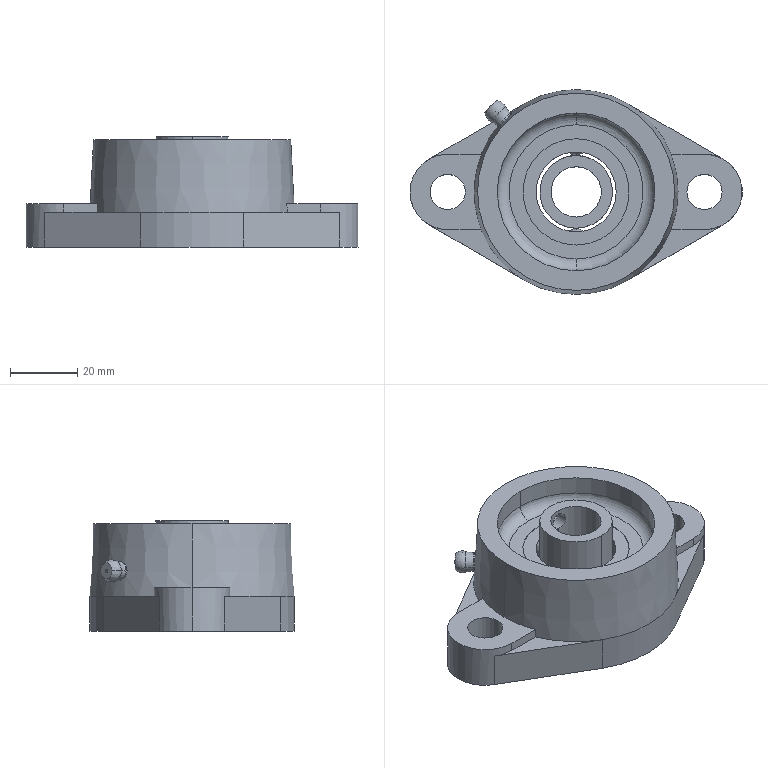Part | SolidWorks | features Revolution 5, Boss 2, RevCut 2, CirPattern 1, Cut 1, Extrusion 1 | 2 solids | 95 faces | box 99 x 61 x 32.9 mm | volume 62248 mm3 | cylinder 44 | plane 33 | sphere 10 | torus 6 | cone 2 | commonest cylinder face diameters 6 x6 22.5 x6 31.72 x6 10.5 x4 23.87 x4 47 x4